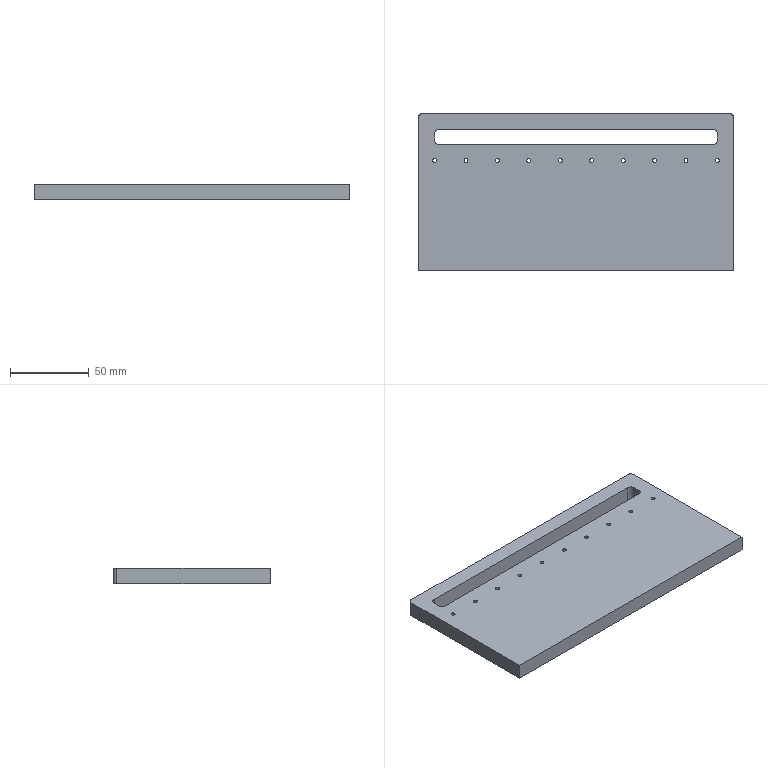Part | STEP file | 001-004-Feeding mechanism shaft slideway vertical plate | 1 solid | 36 faces | box 200 x 100 x 10 mm | volume 181569 mm3 | cylinder 26 | plane 10 | commonest cylinder face diameters 2.5 x20 6 x4 4 x2